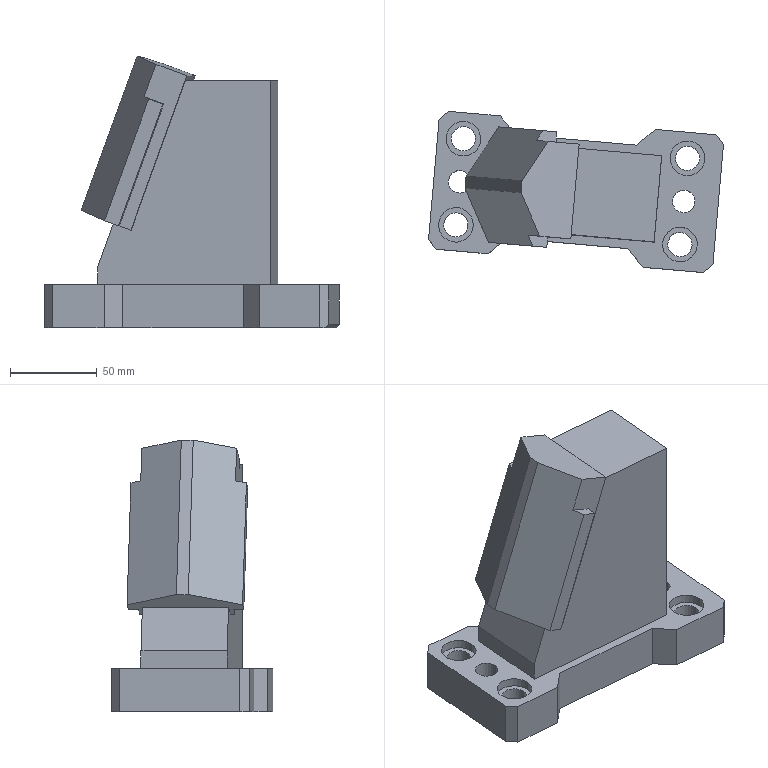Part | NX | features solid 2 | 1 solid | 63 faces | box 170.473 x 93.205 x 157.134 mm | volume 848597 mm3 | plane 43 | cylinder 20 | commonest cylinder face diameters 14 x8 20 x8 13 x4